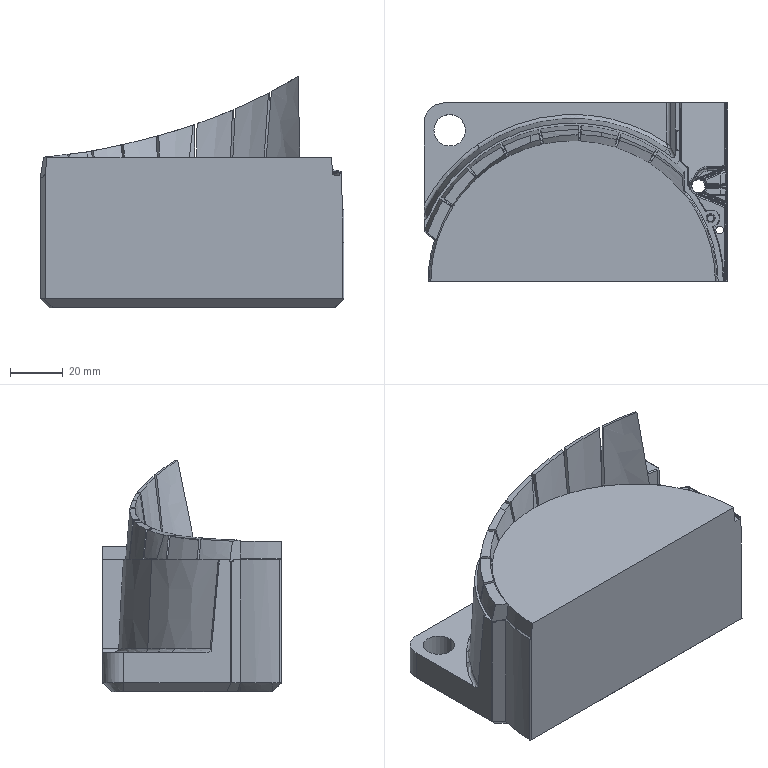Part | Creo | 1 solid | 456 faces | box 115.728 x 68 x 88.268 mm | volume 353598 mm3 | spline 156 | cylinder 116 | plane 82 | cone 57 | sphere 20 | torus 18 | other 7 | commonest cylinder face diameters 0.402 x38 1.005 x19 0.603 x9 16 x7 6.71 x6 8 x6